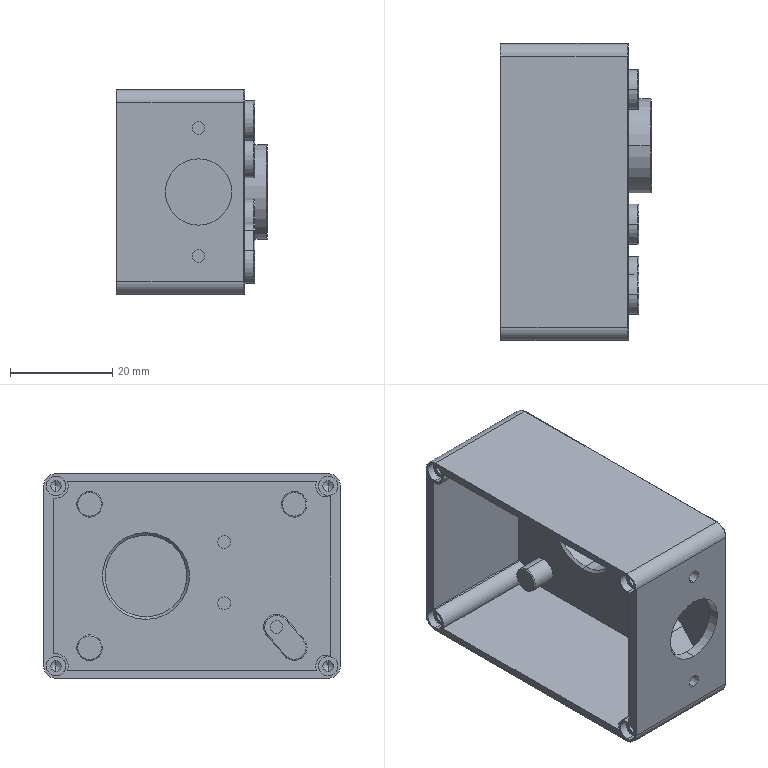Part | SolidWorks | features BaseBody 1 | 1 solid | 160 faces | box 29.528 x 58.024 x 40 mm | volume 12242 mm3 | cylinder 79 | plane 37 | torus 28 | cone 16 | commonest cylinder face diameters 7.8 x14 5 x12 2.5 x10 0.4 x8 2.05 x8 3.3 x8